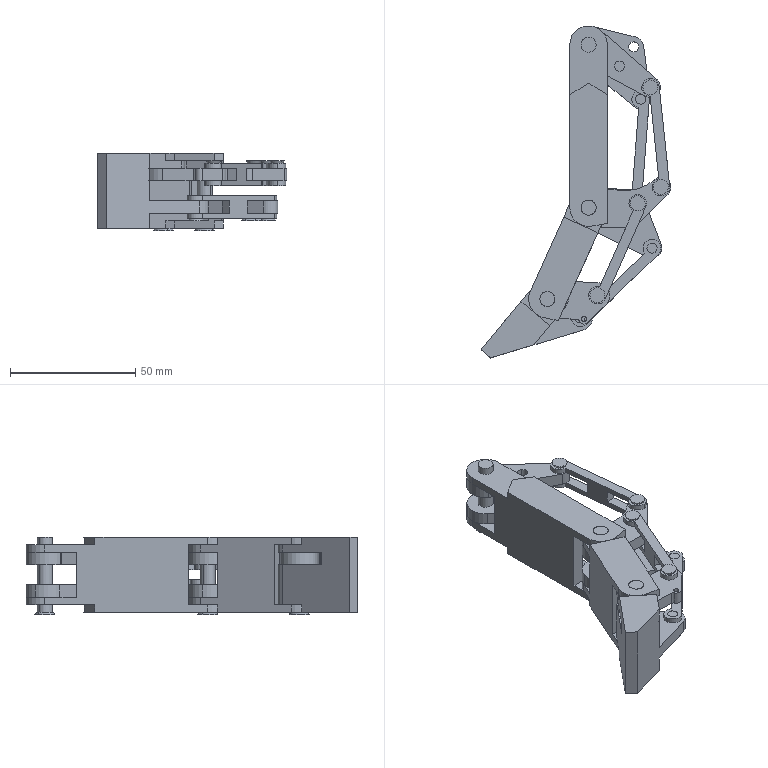Part | SolidWorks | features CompositeCurve 1 | 23 solids | 347 faces | box 75.769 x 132.444 x 31 mm | volume 53046 mm3 | cylinder 167 | plane 158 | cone 22 | commonest cylinder face diameters 4 x69 6 x37 7 x24 15 x19 8 x6 10 x6